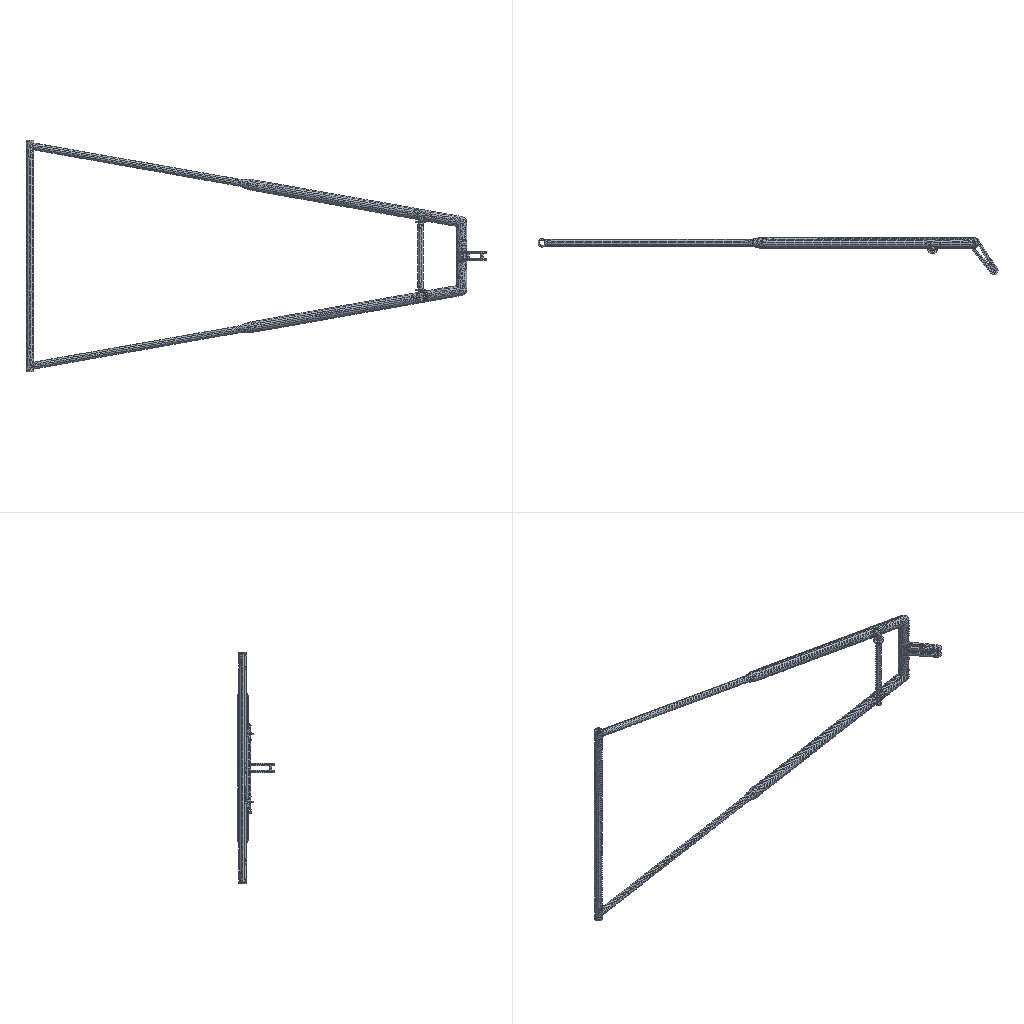Simulation study | ansys workbench
Set-up summary:
category,name,step,type,value,unit,region
solver,ansys_mapdl
solver,version,,,21.1
units,MPA,,stated
analysis,deck,,modal,modal
load_step,requested,,,1
analysis,nlgeom,,,False
mesh,nodes,,,92059
mesh,elements,,,53612
element_type,ANSYS 187 (type 1),,solid,53612
load,load commands in deck,,count,0
bc,support commands in deck,,count,1
named_set,_FIXEDSU,,component
material,1,,in results
check,setup vs results,,match
Ansys APDL input file, long lists of numbers shortened:
/batch
/config,noeldb,1     ! force off writing results to database
*get,_wallstrt,active,,time,wall
! ANSYS input file written by Workbench version 2021 R1
! File used for geometry attach: D:\仿真\受电弓上框架优化分析2026.05.19\模型\skj3(1).STEP
/title,______--__ (C5)
! ****** Begin Custom Load Command Snippet ******
/COM, ACT Extensions:
/COM,     LSDYNA, 2021.1
/COM,
! ****** End   Custom Load Command Snippet ******
*DIM,_wb_ProjectScratch_dir,string,248
_wb_ProjectScratch_dir(1) = 'D:\仿真\受电弓上框架优化分析2026.05.19\_ProjectScratch\Scr4F9D\'
*DIM,_wb_SolverFiles_dir,string,248
_wb_SolverFiles_dir(1) = 'D:\仿真\受电弓上框架优化分析2026.05.19\受电弓上框架_files\dp0\SYS-2\MECH\'
*DIM,_wb_userfiles_dir,string,248
_wb_userfiles_dir(1) = 'D:\仿真\受电弓上框架优化分析2026.05.19\受电弓上框架_files\user_files\'
/com,--- Data in consistent NMM units. See Solving Units in the help system for more information.
/units,MPA
/nopr
/wb,file,start              !  signify a WB generated input file
/prep7
! Turn off shape checking because checks already performed inside WB mesher.
! See help system for more information.
SHPP,OFF,,NOWARN
/nolist
etcon,set             ! allow ANSYS to choose best KEYOP's for 180x elements, resets any applicable keyopt to MAPDL defaults
/com,*********** Nodes for the whole assembly ***********
nblock,3,,101264
(1i9,3e20.9e3)
        1     1.738287455E+03    -2.350226247E+01     3.625000000E+02
! (92058 more lines like these left out)
-1
/wb,elem,start            !  set before creation of elements
/com,*********** Elements for Body 1 "skj3(1)-FreeParts|__-__3" ***********
et,1,187
eblock,19,solid,,53612
(19i9)
        1        1        1        1        0        0        0        0       10        0        1    13475    14341    13639    14333    90244    90732    90239    90242
! (107223 more lines like these left out)
-1
/wb,elem,end               !  done creating elements
/com,*********** Send User Defined Coordinate System(s) ***********
csys,0
toffst,273.15,  ! Temperature offset from absolute zero
/com,*********** Set Reference Temperature ***********
tref,22.
/wb,mat,start              !  starting to send materials
/com,*********** Send Materials ***********
Temperature = 'TEMP' ! Temperature
MP,DENS,1,2.713e-09,	! tonne mm^-3
MP,EX,1,69040,	! tonne s^-2 mm^-1
MP,NUXY,1,0.33,
MP,ALPX,1,2.278e-05,	! C^-1
MP,KXX,1,155.3,	! tonne mm s^-3 C^-1
MP,C,1,915700000,	! mm^2 s^-2 C^-1
/wb,mat,end                !  done sending materials
!************************* Model Summary ********************
!skj3(1)-FreeParts|__-__3,	铝合金，锻造，6061，T6,	matid,	1
!************************* End Model Summary ********************
! get the diagonal of the bounding box. Needed later for other things
*get,_xmin,node,,mnloc,x
*get,_ymin,node,,mnloc,y
*get,_zmin,node,,mnloc,z
*get,_xmax,node,,mxloc,x
*get,_ymax,node,,mxloc,y
*get,_zmax,node,,mxloc,z
_ASMDIAG=(_xmax-_xmin)*(_xmax-_xmin)+(_ymax-_ymin)*(_ymax-_ymin)+(_zmax-_zmin)*(_zmax-_zmin)
_ASMDIAG=SQRT(_ASMDIAG)
/wb,contact,start          !  starting to send contact
/wb,contact,end            !  done creating contacts
/golist
/wb,load,start             !  starting to send loads
/com,*********** Fixed Supports ***********
CMBLOCK,_FIXEDSU,NODE,     5678
(8i10)
       107       108       109       110       111       112       113       114
! (709 more lines like these left out)
cmsel,s,_FIXEDSU
d,all,all
nsel,all
/gst,on,on
fini
*get,_numnode,node,0,count
*get,_numelem,elem,0,count
*get, _MAXELEMNUM, elem, 0, NUM, MAX
*get, _MAXNODENUM, node, 0, NUM, MAX
*get, _MAXELEMTYPE, etyp, 0, NUM, MAX
*get, _MAXREALCONST, real, 0, NUM, MAX
/go
/wb,load,end               !  done creating loads
/com,--- Number of total nodes = %_numnode%
/com,--- Number of contact elements = 0
/com,--- Number of spring elements = 0
/com,--- Number of bearing elements = 0
/com,--- Number of solid elements = 53612
/com,--- Number of condensed parts = 0
/com,--- Number of total elements = %_numelem%
*get,_wallbsol,active,,time,wall
/solu
antype,2                   ! modal analysis
_thickRatio=  1     ! Ratio of thick parts in the model
modopt,lanb,6
outres,erase
outres,all,none
outres,nsol,all
outres,etmp,all
mxpand                    ! default expand in case of complex solution
dmpopt,esav,no
dmpopt,emat,no
dmpopt,full,no
! *********** WB SOLVE COMMAND ***********
! check interactive state
*get,ANSINTER_,active,,int
*if,ANSINTER_,ne,0,then
/eof
*endif
solve
/com *************** Write FE CONNECTORS *********
CEWRITE,file,ce,,INTE
*get,_nmodalsolproc,active,0,numcpu
fini
/nopr
*get,_numnode,node,0,count
*get,_numelem,elem,0,count
*get, _MAXELEMNUM, elem, 0, NUM, MAX
*get, _MAXNODENUM, node, 0, NUM, MAX,,,INTERNAL
*get, _MAXELEMTYPE, etyp, 0, NUM, MAX
*get, _MAXREALCONST, real, 0, NUM, MAX
/gopr
*get,_wallasol,active,,time,wall
/post1
/nopr
*dim,_direction,CHAR,6,1
_direction(1) = 'X'
_direction(2) = 'Y'
_direction(3) = 'Z'
_direction(4) = 'ROTX'
_direction(5) = 'ROTY'
_direction(6) = 'ROTZ'
*get,_lastLS,active,0,set,LSTP
*get,_beginset,active,0,set,nset,first,_lastLS
*get,_endset,active,0,set,nset,last,_lastLS
_nummodes = 0
*if,_endset,gt,0,then
_nummodes = _endset - _beginset + 1
*endif
*do,i_mode,1,_nummodes
   *do,j_component,1,6
			*get,PFACT_%i_mode%_%j_component%,MODE,%i_mode%,PFACT,,DIREC,_direction(%j_component%)
   *enddo
*enddo
*dim,_tmdirection,CHAR,6,1
_tmdirection(1) = 'X'
_tmdirection(2) = 'Y'
_tmdirection(3) = 'Z'
_tmdirection(4) = 'X'
_tmdirection(5) = 'Y'
_tmdirection(6) = 'Z'
*do,j_component,1,6
    *if,j_component,gt,3,then
        *get,TOTALMASS_%j_component%,ELEM,0,IOR,_tmdirection(%j_component%)
    *else
        *get,TOTALMASS_%j_component%,ELEM,0,MTOT,_tmdirection(%j_component%)
    *endif
*enddo
/gopr
xmlo,ENCODING,ISO-8859-1
xmlo,parm
/xml,parm,xml
fini
/gopr
*get,_walldone,active,,time,wall
_preptime=(_wallbsol-_wallstrt)*3600
_solvtime=(_wallasol-_wallbsol)*3600
_posttime=(_walldone-_wallasol)*3600
_totaltim=(_walldone-_wallstrt)*3600
*get,_dlbratio,active,0,solu,dlbr
*get,_combtime,active,0,solu,comb
/com,--- Total number of nodes = %_numnode%
/com,--- Total number of elements = %_numelem%
/com,--- Element load balance ratio = %_dlbratio%
/com,--- Time to combine distributed files = %_combtime%
/wb,file,end               ! done with WB generated input
Results summary:
result,analysis,,,modal
result,last_loadstep,,,1
result,primary field,,,displacement